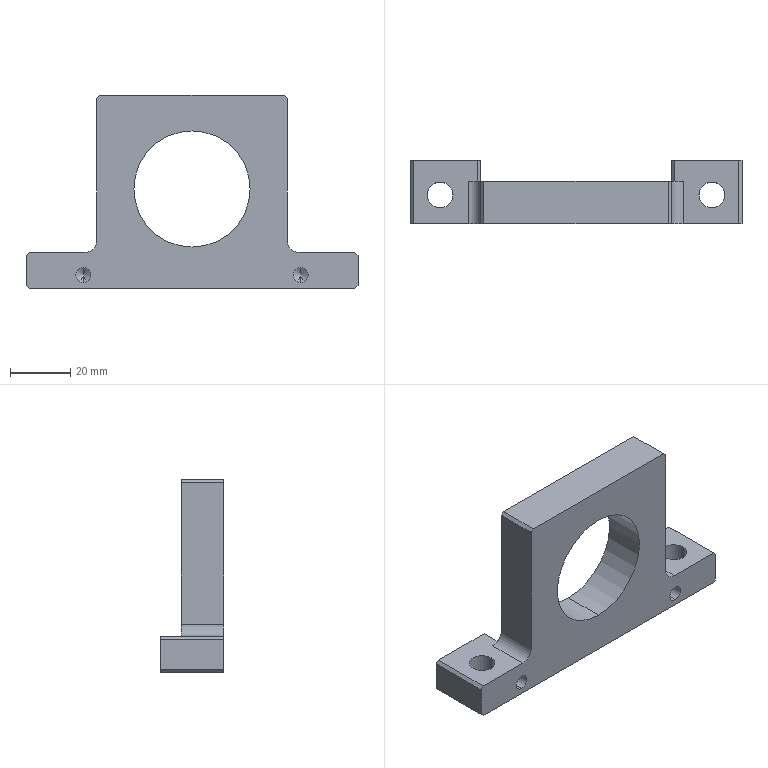Part | STEP file | Motor adapter plate 2 | 1 solid | 56 faces | box 110 x 21 x 64 mm | volume 49771 mm3 | plane 24 | cylinder 20 | cone 12 | commonest cylinder face diameters 3.3 x8 5 x4 8.5 x4 8 x2 38.5 x2